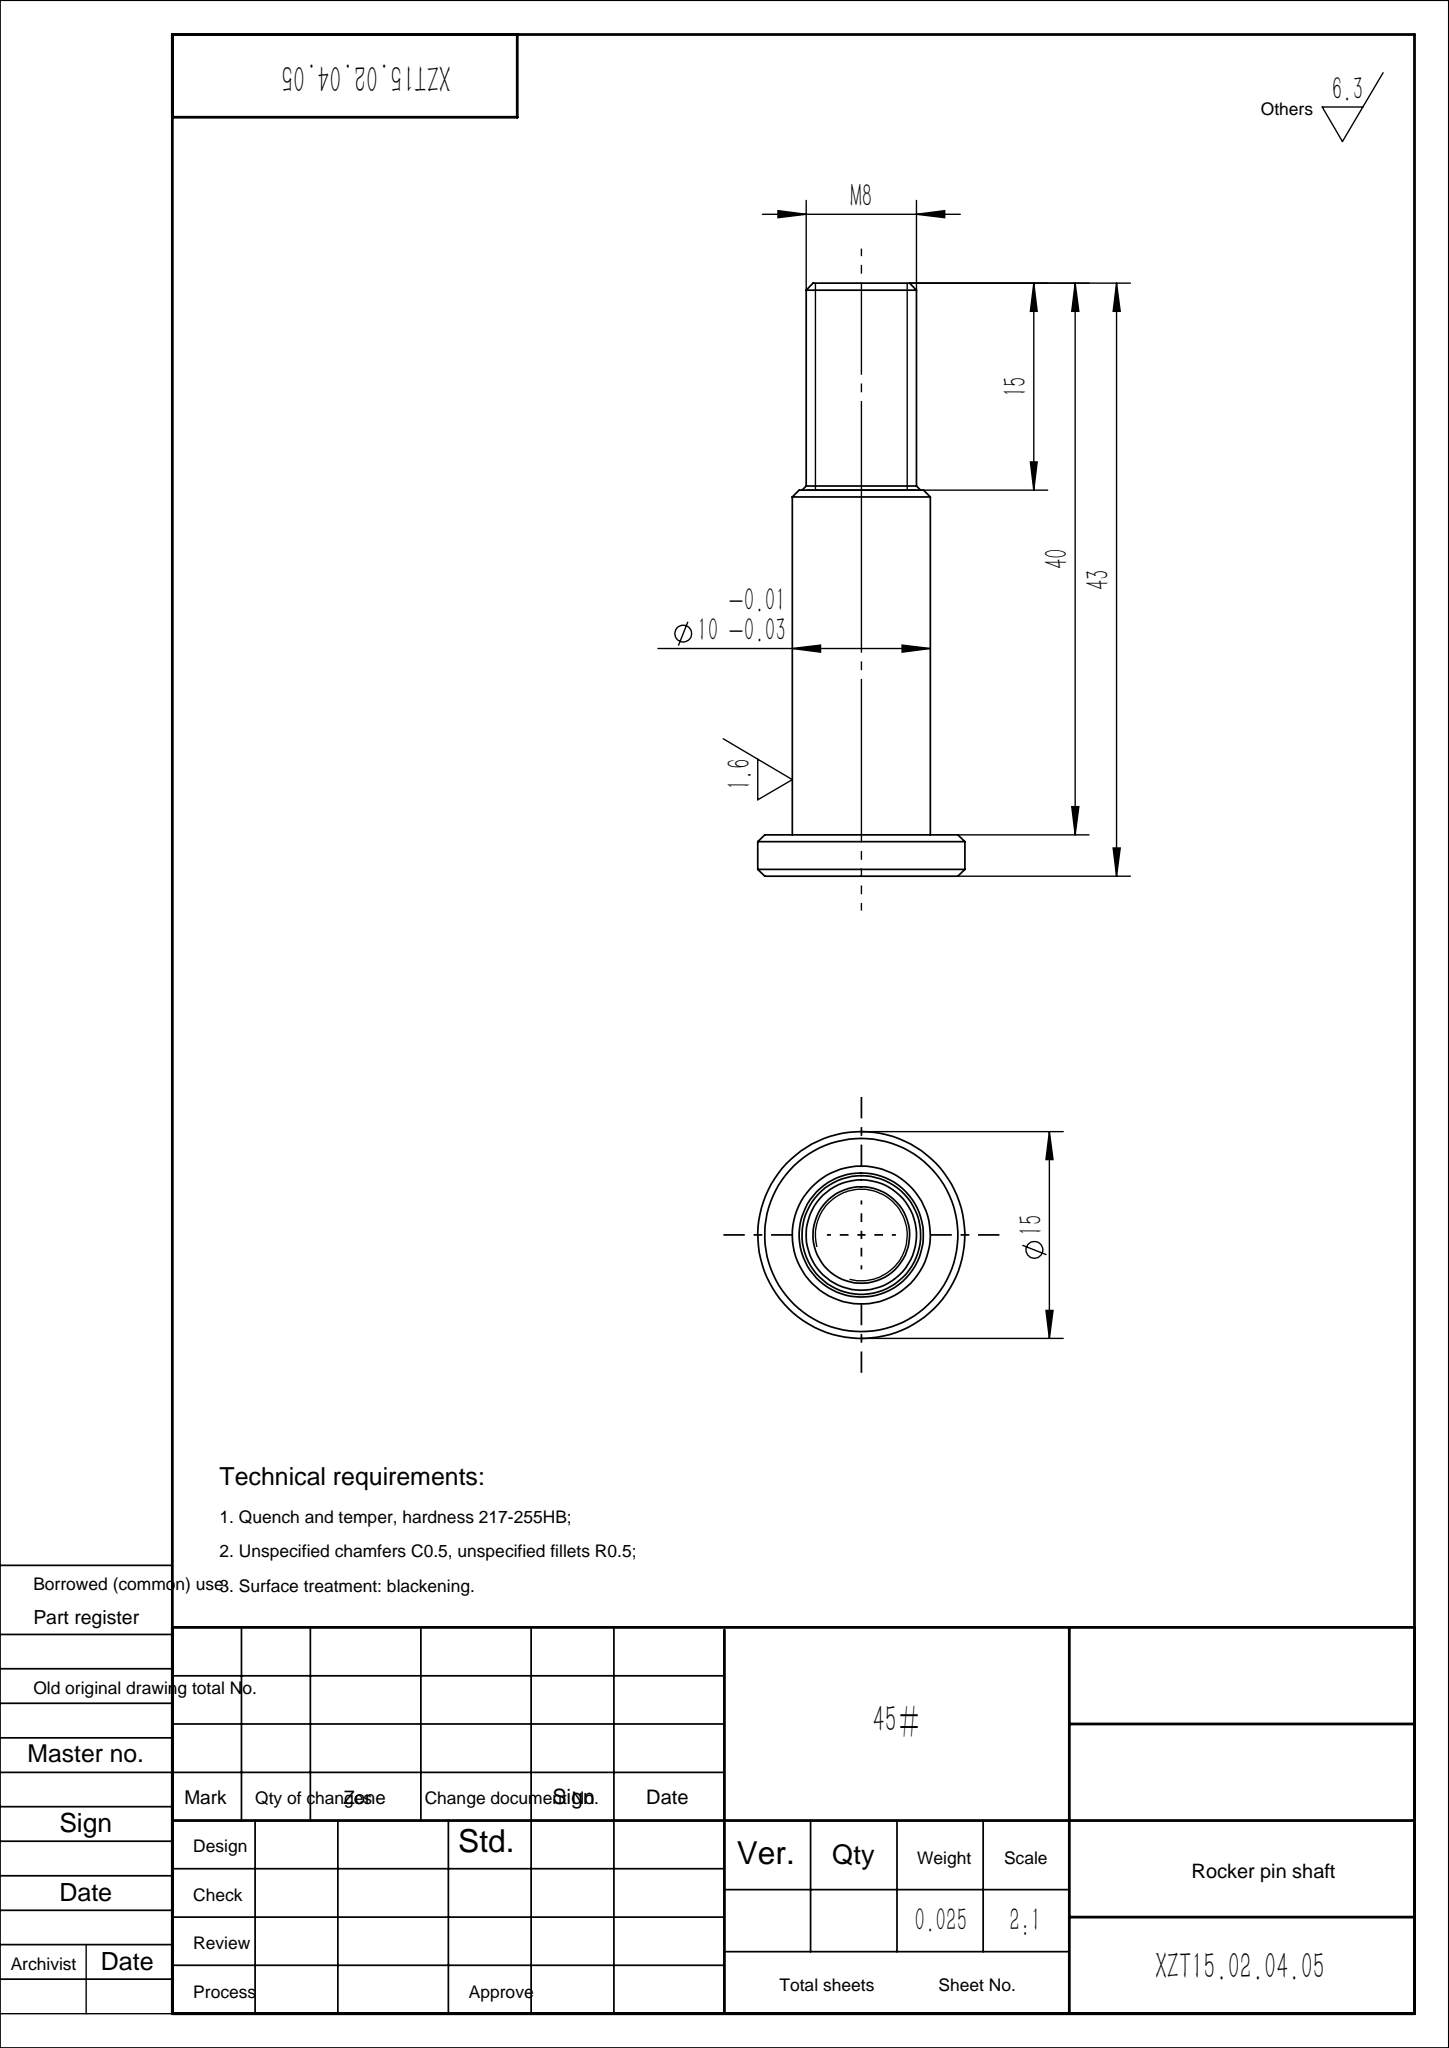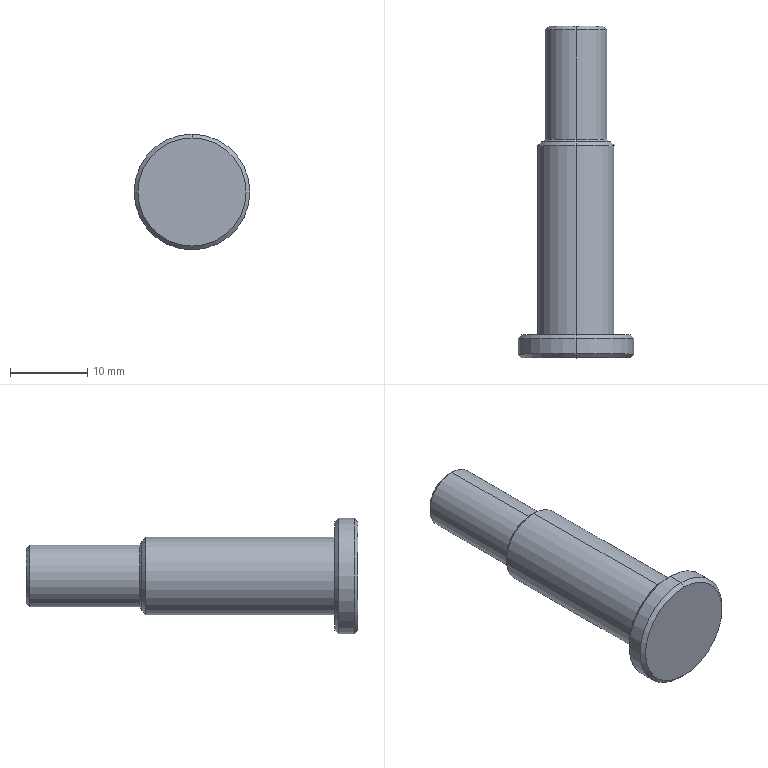Part | SolidWorks | features Chamfer 2, Revolution 1 | 1 solid | 20 faces | box 15 x 43 x 15 mm | volume 3230 mm3 | cone 10 | cylinder 6 | plane 4 | commonest cylinder face diameters 8 x2 10 x2 15 x2
STEP:
#1=CARTESIAN_POINT('',(0.,28.3,4.));
#2=VERTEX_POINT('',#1);
#3=CARTESIAN_POINT('',(0.,28.3,-4.));
#4=VERTEX_POINT('',#3);
#5=CARTESIAN_POINT('',(0.,28.3,0.));
#6=DIRECTION('',(0.,1.,0.));
#7=DIRECTION('',(0.,0.,-1.));
#8=AXIS2_PLACEMENT_3D('',#5,#6,#7);
#9=CIRCLE('',#8,4.);
#10=EDGE_CURVE('',#2,#4,#9,.T.);
#11=ORIENTED_EDGE('',*,*,#10,.F.);
#12=CARTESIAN_POINT('',(0.,28.,4.3));
#13=VERTEX_POINT('',#12);
#14=CARTESIAN_POINT('',(0.,28.3,4.));
#15=DIRECTION('',(0.,-0.7071,0.7071));
#16=VECTOR('',#15,1000.);
#17=LINE('',#14,#16);
#18=EDGE_CURVE('',#2,#13,#17,.T.);
#19=ORIENTED_EDGE('',*,*,#18,.T.);
#20=CARTESIAN_POINT('',(0.,28.,-4.3));
#21=VERTEX_POINT('',#20);
#22=CARTESIAN_POINT('',(0.,28.,0.));
#23=DIRECTION('',(0.,-1.,0.));
#24=DIRECTION('',(0.,0.,-1.));
#25=AXIS2_PLACEMENT_3D('',#22,#23,#24);
#26=CIRCLE('',#25,4.3);
#27=EDGE_CURVE('',#21,#13,#26,.T.);
#28=ORIENTED_EDGE('',*,*,#27,.F.);
#29=CARTESIAN_POINT('',(0.,28.3,-4.));
#30=DIRECTION('',(0.,-0.7071,-0.7071));
#31=VECTOR('',#30,1000.);
#32=LINE('',#29,#31);
#33=EDGE_CURVE('',#4,#21,#32,.T.);
#34=ORIENTED_EDGE('',*,*,#33,.F.);
#35=EDGE_LOOP('',(#11,#19,#28,#34));
#36=FACE_OUTER_BOUND('',#35,.T.);
#37=CARTESIAN_POINT('',(0.,28.3,0.));
#38=DIRECTION('',(0.,-1.,0.));
#39=DIRECTION('',(0.,0.,-1.));
#40=AXIS2_PLACEMENT_3D('',#37,#38,#39);
#41=CONICAL_SURFACE('',#40,4.,0.7854);
#42=ADVANCED_FACE('',(#36),#41,.T.);
#43=CARTESIAN_POINT('',(0.,28.,4.5));
#44=VERTEX_POINT('',#43);
#45=CARTESIAN_POINT('',(0.,28.,-4.5));
#46=VERTEX_POINT('',#45);
#47=CARTESIAN_POINT('',(0.,28.,0.));
#48=DIRECTION('',(0.,1.,0.));
#49=DIRECTION('',(0.,0.,-1.));
#50=AXIS2_PLACEMENT_3D('',#47,#48,#49);
#51=CIRCLE('',#50,4.5);
#52=EDGE_CURVE('',#44,#46,#51,.T.);
#53=ORIENTED_EDGE('',*,*,#52,.F.);
#54=CARTESIAN_POINT('',(0.,27.5,5.));
#55=VERTEX_POINT('',#54);
#56=CARTESIAN_POINT('',(0.,28.,4.5));
#57=DIRECTION('',(0.,-0.7071,0.7071));
#58=VECTOR('',#57,1000.);
#59=LINE('',#56,#58);
#60=EDGE_CURVE('',#44,#55,#59,.T.);
#61=ORIENTED_EDGE('',*,*,#60,.T.);
#62=CARTESIAN_POINT('',(0.,27.5,-5.));
#63=VERTEX_POINT('',#62);
#64=CARTESIAN_POINT('',(0.,27.5,0.));
#65=DIRECTION('',(0.,-1.,0.));
#66=DIRECTION('',(0.,0.,-1.));
#67=AXIS2_PLACEMENT_3D('',#64,#65,#66);
#68=CIRCLE('',#67,5.);
#69=EDGE_CURVE('',#63,#55,#68,.T.);
#70=ORIENTED_EDGE('',*,*,#69,.F.);
#71=CARTESIAN_POINT('',(0.,28.,-4.5));
#72=DIRECTION('',(0.,-0.7071,-0.7071));
#73=VECTOR('',#72,1000.);
#74=LINE('',#71,#73);
#75=EDGE_CURVE('',#46,#63,#74,.T.);
#76=ORIENTED_EDGE('',*,*,#75,.F.);
#77=EDGE_LOOP('',(#53,#61,#70,#76));
#78=FACE_OUTER_BOUND('',#77,.T.);
#79=CARTESIAN_POINT('',(0.,28.,0.));
#80=DIRECTION('',(0.,-1.,0.));
#81=DIRECTION('',(0.,0.,-1.));
#82=AXIS2_PLACEMENT_3D('',#79,#80,#81);
#83=CONICAL_SURFACE('',#82,4.5,0.7854);
#84=ADVANCED_FACE('',(#78),#83,.T.);
#85=CARTESIAN_POINT('',(0.,0.,-7.));
#86=VERTEX_POINT('',#85);
#87=CARTESIAN_POINT('',(0.,0.,7.));
#88=VERTEX_POINT('',#87);
#89=CARTESIAN_POINT('',(0.,0.,0.));
#90=DIRECTION('',(0.,-1.,0.));
#91=DIRECTION('',(0.,0.,1.));
#92=AXIS2_PLACEMENT_3D('',#89,#90,#91);
#93=CIRCLE('',#92,7.);
#94=EDGE_CURVE('',#86,#88,#93,.T.);
#95=ORIENTED_EDGE('',*,*,#94,.F.);
#96=CARTESIAN_POINT('',(0.,0.5,-7.5));
#97=VERTEX_POINT('',#96);
#98=CARTESIAN_POINT('',(0.,0.5,-7.5));
#99=DIRECTION('',(0.,0.7071,-0.7071));
#100=VECTOR('',#99,1000.);
#101=LINE('',#98,#100);
#102=EDGE_CURVE('',#86,#97,#101,.T.);
#103=ORIENTED_EDGE('',*,*,#102,.T.);
#104=CARTESIAN_POINT('',(0.,0.5,7.5));
#105=VERTEX_POINT('',#104);
#106=CARTESIAN_POINT('',(0.,0.5,0.));
#107=DIRECTION('',(0.,1.,0.));
#108=DIRECTION('',(0.,0.,1.));
#109=AXIS2_PLACEMENT_3D('',#106,#107,#108);
#110=CIRCLE('',#109,7.5);
#111=EDGE_CURVE('',#105,#97,#110,.T.);
#112=ORIENTED_EDGE('',*,*,#111,.F.);
#113=CARTESIAN_POINT('',(0.,0.5,7.5));
#114=DIRECTION('',(0.,0.7071,0.7071));
#115=VECTOR('',#114,1000.);
#116=LINE('',#113,#115);
#117=EDGE_CURVE('',#88,#105,#116,.T.);
#118=ORIENTED_EDGE('',*,*,#117,.F.);
#119=EDGE_LOOP('',(#95,#103,#112,#118));
#120=FACE_OUTER_BOUND('',#119,.T.);
#121=CARTESIAN_POINT('',(0.,0.5,0.));
#122=DIRECTION('',(0.,1.,0.));
#123=DIRECTION('',(0.,0.,1.));
#124=AXIS2_PLACEMENT_3D('',#121,#122,#123);
#125=CONICAL_SURFACE('',#124,7.5,0.7854);
#126=ADVANCED_FACE('',(#120),#125,.T.);
#127=CARTESIAN_POINT('',(0.,3.,7.));
#128=VERTEX_POINT('',#127);
#129=CARTESIAN_POINT('',(0.,3.,-7.));
#130=VERTEX_POINT('',#129);
#131=CARTESIAN_POINT('',(0.,3.,0.));
#132=DIRECTION('',(0.,1.,0.));
#133=DIRECTION('',(0.,0.,-1.));
#134=AXIS2_PLACEMENT_3D('',#131,#132,#133);
#135=CIRCLE('',#134,7.);
#136=EDGE_CURVE('',#128,#130,#135,.T.);
#137=ORIENTED_EDGE('',*,*,#136,.F.);
#138=CARTESIAN_POINT('',(0.,2.5,7.5));
#139=VERTEX_POINT('',#138);
#140=CARTESIAN_POINT('',(0.,3.,7.));
#141=DIRECTION('',(0.,-0.7071,0.7071));
#142=VECTOR('',#141,1000.);
#143=LINE('',#140,#142);
#144=EDGE_CURVE('',#128,#139,#143,.T.);
#145=ORIENTED_EDGE('',*,*,#144,.T.);
#146=CARTESIAN_POINT('',(0.,2.5,-7.5));
#147=VERTEX_POINT('',#146);
#148=CARTESIAN_POINT('',(0.,2.5,0.));
#149=DIRECTION('',(0.,-1.,0.));
#150=DIRECTION('',(0.,0.,-1.));
#151=AXIS2_PLACEMENT_3D('',#148,#149,#150);
#152=CIRCLE('',#151,7.5);
#153=EDGE_CURVE('',#147,#139,#152,.T.);
#154=ORIENTED_EDGE('',*,*,#153,.F.);
#155=CARTESIAN_POINT('',(0.,3.,-7.));
#156=DIRECTION('',(0.,-0.7071,-0.7071));
#157=VECTOR('',#156,1000.);
#158=LINE('',#155,#157);
#159=EDGE_CURVE('',#130,#147,#158,.T.);
#160=ORIENTED_EDGE('',*,*,#159,.F.);
#161=EDGE_LOOP('',(#137,#145,#154,#160));
#162=FACE_OUTER_BOUND('',#161,.T.);
#163=CARTESIAN_POINT('',(0.,3.,0.));
#164=DIRECTION('',(0.,-1.,0.));
#165=DIRECTION('',(0.,0.,-1.));
#166=AXIS2_PLACEMENT_3D('',#163,#164,#165);
#167=CONICAL_SURFACE('',#166,7.,0.7854);
#168=ADVANCED_FACE('',(#162),#167,.T.);
#169=CARTESIAN_POINT('',(0.,43.,3.5));
#170=VERTEX_POINT('',#169);
#171=CARTESIAN_POINT('',(0.,43.,-3.5));
#172=VERTEX_POINT('',#171);
#173=CARTESIAN_POINT('',(0.,43.,0.));
#174=DIRECTION('',(0.,1.,0.));
#175=DIRECTION('',(0.,0.,-1.));
#176=AXIS2_PLACEMENT_3D('',#173,#174,#175);
#177=CIRCLE('',#176,3.5);
#178=EDGE_CURVE('',#170,#172,#177,.T.);
#179=ORIENTED_EDGE('',*,*,#178,.F.);
#180=CARTESIAN_POINT('',(0.,42.5,4.));
#181=VERTEX_POINT('',#180);
#182=CARTESIAN_POINT('',(0.,43.,3.5));
#183=DIRECTION('',(0.,-0.7071,0.7071));
#184=VECTOR('',#183,1000.);
#185=LINE('',#182,#184);
#186=EDGE_CURVE('',#170,#181,#185,.T.);
#187=ORIENTED_EDGE('',*,*,#186,.T.);
#188=CARTESIAN_POINT('',(0.,42.5,-4.));
#189=VERTEX_POINT('',#188);
#190=CARTESIAN_POINT('',(0.,42.5,0.));
#191=DIRECTION('',(0.,-1.,0.));
#192=DIRECTION('',(0.,0.,-1.));
#193=AXIS2_PLACEMENT_3D('',#190,#191,#192);
#194=CIRCLE('',#193,4.);
#195=EDGE_CURVE('',#189,#181,#194,.T.);
#196=ORIENTED_EDGE('',*,*,#195,.F.);
#197=CARTESIAN_POINT('',(0.,43.,-3.5));
#198=DIRECTION('',(0.,-0.7071,-0.7071));
#199=VECTOR('',#198,1000.);
#200=LINE('',#197,#199);
#201=EDGE_CURVE('',#172,#189,#200,.T.);
#202=ORIENTED_EDGE('',*,*,#201,.F.);
#203=EDGE_LOOP('',(#179,#187,#196,#202));
#204=FACE_OUTER_BOUND('',#203,.T.);
#205=CARTESIAN_POINT('',(0.,43.,0.));
#206=DIRECTION('',(0.,-1.,0.));
#207=DIRECTION('',(0.,0.,-1.));
#208=AXIS2_PLACEMENT_3D('',#205,#206,#207);
#209=CONICAL_SURFACE('',#208,3.5,0.7854);
#210=ADVANCED_FACE('',(#204),#209,.T.);
#211=ORIENTED_EDGE('',*,*,#10,.T.);
#212=CARTESIAN_POINT('',(0.,0.,-4.));
#213=DIRECTION('',(0.,1.,0.));
#214=VECTOR('',#213,1000.);
#215=LINE('',#212,#214);
#216=EDGE_CURVE('',#4,#189,#215,.T.);
#217=ORIENTED_EDGE('',*,*,#216,.T.);
#218=ORIENTED_EDGE('',*,*,#195,.T.);
#219=CARTESIAN_POINT('',(0.,0.,4.));
#220=DIRECTION('',(0.,1.,0.));
#221=VECTOR('',#220,1000.);
#222=LINE('',#219,#221);
#223=EDGE_CURVE('',#2,#181,#222,.T.);
#224=ORIENTED_EDGE('',*,*,#223,.F.);
#225=EDGE_LOOP('',(#211,#217,#218,#224));
#226=FACE_OUTER_BOUND('',#225,.T.);
#227=CARTESIAN_POINT('',(0.,0.,0.));
#228=DIRECTION('',(0.,1.,0.));
#229=DIRECTION('',(0.,0.,1.));
#230=AXIS2_PLACEMENT_3D('',#227,#228,#229);
#231=CYLINDRICAL_SURFACE('',#230,4.);
#232=ADVANCED_FACE('',(#226),#231,.T.);
#233=CARTESIAN_POINT('',(0.,3.,5.));
#234=VERTEX_POINT('',#233);
#235=CARTESIAN_POINT('',(0.,3.,-5.));
#236=VERTEX_POINT('',#235);
#237=CARTESIAN_POINT('',(0.,3.,0.));
#238=DIRECTION('',(0.,1.,0.));
#239=DIRECTION('',(0.,0.,1.));
#240=AXIS2_PLACEMENT_3D('',#237,#238,#239);
#241=CIRCLE('',#240,5.);
#242=EDGE_CURVE('',#234,#236,#241,.T.);
#243=ORIENTED_EDGE('',*,*,#242,.T.);
#244=CARTESIAN_POINT('',(0.,0.,-5.));
#245=DIRECTION('',(0.,1.,0.));
#246=VECTOR('',#245,1000.);
#247=LINE('',#244,#246);
#248=EDGE_CURVE('',#236,#63,#247,.T.);
#249=ORIENTED_EDGE('',*,*,#248,.T.);
#250=ORIENTED_EDGE('',*,*,#69,.T.);
#251=CARTESIAN_POINT('',(0.,0.,5.));
#252=DIRECTION('',(0.,1.,0.));
#253=VECTOR('',#252,1000.);
#254=LINE('',#251,#253);
#255=EDGE_CURVE('',#234,#55,#254,.T.);
#256=ORIENTED_EDGE('',*,*,#255,.F.);
#257=EDGE_LOOP('',(#243,#249,#250,#256));
#258=FACE_OUTER_BOUND('',#257,.T.);
#259=CARTESIAN_POINT('',(0.,0.,0.));
#260=DIRECTION('',(0.,1.,0.));
#261=DIRECTION('',(0.,0.,1.));
#262=AXIS2_PLACEMENT_3D('',#259,#260,#261);
#263=CYLINDRICAL_SURFACE('',#262,5.);
#264=ADVANCED_FACE('',(#258),#263,.T.);
#265=ORIENTED_EDGE('',*,*,#111,.T.);
#266=CARTESIAN_POINT('',(0.,0.,-7.5));
#267=DIRECTION('',(0.,1.,0.));
#268=VECTOR('',#267,1000.);
#269=LINE('',#266,#268);
#270=EDGE_CURVE('',#97,#147,#269,.T.);
#271=ORIENTED_EDGE('',*,*,#270,.T.);
#272=ORIENTED_EDGE('',*,*,#153,.T.);
#273=CARTESIAN_POINT('',(0.,0.,7.5));
#274=DIRECTION('',(0.,1.,0.));
#275=VECTOR('',#274,1000.);
#276=LINE('',#273,#275);
#277=EDGE_CURVE('',#105,#139,#276,.T.);
#278=ORIENTED_EDGE('',*,*,#277,.F.);
#279=EDGE_LOOP('',(#265,#271,#272,#278));
#280=FACE_OUTER_BOUND('',#279,.T.);
#281=CARTESIAN_POINT('',(0.,0.,0.));
#282=DIRECTION('',(0.,1.,0.));
#283=DIRECTION('',(0.,0.,1.));
#284=AXIS2_PLACEMENT_3D('',#281,#282,#283);
#285=CYLINDRICAL_SURFACE('',#284,7.5);
#286=ADVANCED_FACE('',(#280),#285,.T.);
#287=CARTESIAN_POINT('',(0.,0.,0.));
#288=DIRECTION('',(0.,-1.,0.));
#289=DIRECTION('',(0.,0.,1.));
#290=AXIS2_PLACEMENT_3D('',#287,#288,#289);
#291=CIRCLE('',#290,7.);
#292=EDGE_CURVE('',#88,#86,#291,.T.);
#293=ORIENTED_EDGE('',*,*,#292,.T.);
#294=ORIENTED_EDGE('',*,*,#94,.T.);
#295=EDGE_LOOP('',(#293,#294));
#296=FACE_OUTER_BOUND('',#295,.T.);
#297=CARTESIAN_POINT('',(0.,0.,0.));
#298=DIRECTION('',(0.,1.,0.));
#299=DIRECTION('',(0.,0.,1.));
#300=AXIS2_PLACEMENT_3D('',#297,#298,#299);
#301=PLANE('',#300);
#302=ADVANCED_FACE('',(#296),#301,.F.);
#303=ORIENTED_EDGE('',*,*,#270,.F.);
#304=CARTESIAN_POINT('',(0.,0.5,0.));
#305=DIRECTION('',(0.,1.,0.));
#306=DIRECTION('',(0.,0.,1.));
#307=AXIS2_PLACEMENT_3D('',#304,#305,#306);
#308=CIRCLE('',#307,7.5);
#309=EDGE_CURVE('',#97,#105,#308,.T.);
#310=ORIENTED_EDGE('',*,*,#309,.T.);
#311=ORIENTED_EDGE('',*,*,#277,.T.);
#312=CARTESIAN_POINT('',(0.,2.5,0.));
#313=DIRECTION('',(0.,-1.,0.));
#314=DIRECTION('',(0.,0.,-1.));
#315=AXIS2_PLACEMENT_3D('',#312,#313,#314);
#316=CIRCLE('',#315,7.5);
#317=EDGE_CURVE('',#139,#147,#316,.T.);
#318=ORIENTED_EDGE('',*,*,#317,.T.);
#319=EDGE_LOOP('',(#303,#310,#311,#318));
#320=FACE_OUTER_BOUND('',#319,.T.);
#321=CARTESIAN_POINT('',(0.,0.,0.));
#322=DIRECTION('',(0.,1.,0.));
#323=DIRECTION('',(0.,0.,1.));
#324=AXIS2_PLACEMENT_3D('',#321,#322,#323);
#325=CYLINDRICAL_SURFACE('',#324,7.5);
#326=ADVANCED_FACE('',(#320),#325,.T.);
#327=CARTESIAN_POINT('',(0.,3.,0.));
#328=DIRECTION('',(0.,1.,0.));
#329=DIRECTION('',(0.,0.,-1.));
#330=AXIS2_PLACEMENT_3D('',#327,#328,#329);
#331=CIRCLE('',#330,7.);
#332=EDGE_CURVE('',#130,#128,#331,.T.);
#333=ORIENTED_EDGE('',*,*,#332,.T.);
#334=ORIENTED_EDGE('',*,*,#136,.T.);
#335=EDGE_LOOP('',(#333,#334));
#336=FACE_OUTER_BOUND('',#335,.T.);
#337=ORIENTED_EDGE('',*,*,#242,.F.);
#338=CARTESIAN_POINT('',(0.,3.,0.));
#339=DIRECTION('',(0.,1.,0.));
#340=DIRECTION('',(0.,0.,1.));
#341=AXIS2_PLACEMENT_3D('',#338,#339,#340);
#342=CIRCLE('',#341,5.);
#343=EDGE_CURVE('',#236,#234,#342,.T.);
#344=ORIENTED_EDGE('',*,*,#343,.F.);
#345=EDGE_LOOP('',(#337,#344));
#346=FACE_BOUND('',#345,.T.);
#347=CARTESIAN_POINT('',(7.5,3.,0.));
#348=DIRECTION('',(0.,-1.,0.));
#349=DIRECTION('',(0.,0.,-1.));
#350=AXIS2_PLACEMENT_3D('',#347,#348,#349);
#351=PLANE('',#350);
#352=ADVANCED_FACE('',(#336,#346),#351,.F.);
#353=ORIENTED_EDGE('',*,*,#248,.F.);
#354=ORIENTED_EDGE('',*,*,#343,.T.);
#355=ORIENTED_EDGE('',*,*,#255,.T.);
#356=CARTESIAN_POINT('',(0.,27.5,0.));
#357=DIRECTION('',(0.,-1.,0.));
#358=DIRECTION('',(0.,0.,-1.));
#359=AXIS2_PLACEMENT_3D('',#356,#357,#358);
#360=CIRCLE('',#359,5.);
#361=EDGE_CURVE('',#55,#63,#360,.T.);
#362=ORIENTED_EDGE('',*,*,#361,.T.);
#363=EDGE_LOOP('',(#353,#354,#355,#362));
#364=FACE_OUTER_BOUND('',#363,.T.);
#365=CARTESIAN_POINT('',(0.,0.,0.));
#366=DIRECTION('',(0.,1.,0.));
#367=DIRECTION('',(0.,0.,1.));
#368=AXIS2_PLACEMENT_3D('',#365,#366,#367);
#369=CYLINDRICAL_SURFACE('',#368,5.);
#370=ADVANCED_FACE('',(#364),#369,.T.);
#371=ORIENTED_EDGE('',*,*,#27,.T.);
#372=CARTESIAN_POINT('',(0.,28.,0.));
#373=DIRECTION('',(0.,-1.,0.));
#374=DIRECTION('',(0.,0.,-1.));
#375=AXIS2_PLACEMENT_3D('',#372,#373,#374);
#376=CIRCLE('',#375,4.3);
#377=EDGE_CURVE('',#13,#21,#376,.T.);
#378=ORIENTED_EDGE('',*,*,#377,.T.);
#379=EDGE_LOOP('',(#371,#378));
#380=FACE_BOUND('',#379,.T.);
#381=CARTESIAN_POINT('',(0.,28.,0.));
#382=DIRECTION('',(0.,1.,0.));
#383=DIRECTION('',(0.,0.,-1.));
#384=AXIS2_PLACEMENT_3D('',#381,#382,#383);
#385=CIRCLE('',#384,4.5);
#386=EDGE_CURVE('',#46,#44,#385,.T.);
#387=ORIENTED_EDGE('',*,*,#386,.T.);
#388=ORIENTED_EDGE('',*,*,#52,.T.);
#389=EDGE_LOOP('',(#387,#388));
#390=FACE_OUTER_BOUND('',#389,.T.);
#391=CARTESIAN_POINT('',(5.,28.,0.));
#392=DIRECTION('',(0.,-1.,0.));
#393=DIRECTION('',(0.,0.,-1.));
#394=AXIS2_PLACEMENT_3D('',#391,#392,#393);
#395=PLANE('',#394);
#396=ADVANCED_FACE('',(#380,#390),#395,.F.);
#397=ORIENTED_EDGE('',*,*,#216,.F.);
#398=CARTESIAN_POINT('',(0.,28.3,0.));
#399=DIRECTION('',(0.,1.,0.));
#400=DIRECTION('',(0.,0.,-1.));
#401=AXIS2_PLACEMENT_3D('',#398,#399,#400);
#402=CIRCLE('',#401,4.);
#403=EDGE_CURVE('',#4,#2,#402,.T.);
#404=ORIENTED_EDGE('',*,*,#403,.T.);
#405=ORIENTED_EDGE('',*,*,#223,.T.);
#406=CARTESIAN_POINT('',(0.,42.5,0.));
#407=DIRECTION('',(0.,-1.,0.));
#408=DIRECTION('',(0.,0.,-1.));
#409=AXIS2_PLACEMENT_3D('',#406,#407,#408);
#410=CIRCLE('',#409,4.);
#411=EDGE_CURVE('',#181,#189,#410,.T.);
#412=ORIENTED_EDGE('',*,*,#411,.T.);
#413=EDGE_LOOP('',(#397,#404,#405,#412));
#414=FACE_OUTER_BOUND('',#413,.T.);
#415=CARTESIAN_POINT('',(0.,0.,0.));
#416=DIRECTION('',(0.,1.,0.));
#417=DIRECTION('',(0.,0.,1.));
#418=AXIS2_PLACEMENT_3D('',#415,#416,#417);
#419=CYLINDRICAL_SURFACE('',#418,4.);
#420=ADVANCED_FACE('',(#414),#419,.T.);
#421=CARTESIAN_POINT('',(0.,43.,0.));
#422=DIRECTION('',(0.,1.,0.));
#423=DIRECTION('',(0.,0.,-1.));
#424=AXIS2_PLACEMENT_3D('',#421,#422,#423);
#425=CIRCLE('',#424,3.5);
#426=EDGE_CURVE('',#172,#170,#425,.T.);
#427=ORIENTED_EDGE('',*,*,#426,.T.);
#428=ORIENTED_EDGE('',*,*,#178,.T.);
#429=EDGE_LOOP('',(#427,#428));
#430=FACE_OUTER_BOUND('',#429,.T.);
#431=CARTESIAN_POINT('',(4.,43.,0.));
#432=DIRECTION('',(0.,-1.,0.));
#433=DIRECTION('',(0.,0.,-1.));
#434=AXIS2_PLACEMENT_3D('',#431,#432,#433);
#435=PLANE('',#434);
#436=ADVANCED_FACE('',(#430),#435,.F.);
#437=ORIENTED_EDGE('',*,*,#186,.F.);
#438=ORIENTED_EDGE('',*,*,#426,.F.);
#439=ORIENTED_EDGE('',*,*,#201,.T.);
#440=ORIENTED_EDGE('',*,*,#411,.F.);
#441=EDGE_LOOP('',(#437,#438,#439,#440));
#442=FACE_OUTER_BOUND('',#441,.T.);
#443=CARTESIAN_POINT('',(0.,43.,0.));
#444=DIRECTION('',(0.,-1.,0.));
#445=DIRECTION('',(0.,0.,-1.));
#446=AXIS2_PLACEMENT_3D('',#443,#444,#445);
#447=CONICAL_SURFACE('',#446,3.5,0.7854);
#448=ADVANCED_FACE('',(#442),#447,.T.);
#449=ORIENTED_EDGE('',*,*,#144,.F.);
#450=ORIENTED_EDGE('',*,*,#332,.F.);
#451=ORIENTED_EDGE('',*,*,#159,.T.);
#452=ORIENTED_EDGE('',*,*,#317,.F.);
#453=EDGE_LOOP('',(#449,#450,#451,#452));
#454=FACE_OUTER_BOUND('',#453,.T.);
#455=CARTESIAN_POINT('',(0.,3.,0.));
#456=DIRECTION('',(0.,-1.,0.));
#457=DIRECTION('',(0.,0.,-1.));
#458=AXIS2_PLACEMENT_3D('',#455,#456,#457);
#459=CONICAL_SURFACE('',#458,7.,0.7854);
#460=ADVANCED_FACE('',(#454),#459,.T.);
#461=ORIENTED_EDGE('',*,*,#102,.F.);
#462=ORIENTED_EDGE('',*,*,#292,.F.);
#463=ORIENTED_EDGE('',*,*,#117,.T.);
#464=ORIENTED_EDGE('',*,*,#309,.F.);
#465=EDGE_LOOP('',(#461,#462,#463,#464));
#466=FACE_OUTER_BOUND('',#465,.T.);
#467=CARTESIAN_POINT('',(0.,0.5,0.));
#468=DIRECTION('',(0.,1.,0.));
#469=DIRECTION('',(0.,0.,1.));
#470=AXIS2_PLACEMENT_3D('',#467,#468,#469);
#471=CONICAL_SURFACE('',#470,7.5,0.7854);
#472=ADVANCED_FACE('',(#466),#471,.T.);
#473=ORIENTED_EDGE('',*,*,#60,.F.);
#474=ORIENTED_EDGE('',*,*,#386,.F.);
#475=ORIENTED_EDGE('',*,*,#75,.T.);
#476=ORIENTED_EDGE('',*,*,#361,.F.);
#477=EDGE_LOOP('',(#473,#474,#475,#476));
#478=FACE_OUTER_BOUND('',#477,.T.);
#479=CARTESIAN_POINT('',(0.,28.,0.));
#480=DIRECTION('',(0.,-1.,0.));
#481=DIRECTION('',(0.,0.,-1.));
#482=AXIS2_PLACEMENT_3D('',#479,#480,#481);
#483=CONICAL_SURFACE('',#482,4.5,0.7854);
#484=ADVANCED_FACE('',(#478),#483,.T.);
#485=ORIENTED_EDGE('',*,*,#18,.F.);
#486=ORIENTED_EDGE('',*,*,#403,.F.);
#487=ORIENTED_EDGE('',*,*,#33,.T.);
#488=ORIENTED_EDGE('',*,*,#377,.F.);
#489=EDGE_LOOP('',(#485,#486,#487,#488));
#490=FACE_OUTER_BOUND('',#489,.T.);
#491=CARTESIAN_POINT('',(0.,28.3,0.));
#492=DIRECTION('',(0.,-1.,0.));
#493=DIRECTION('',(0.,0.,-1.));
#494=AXIS2_PLACEMENT_3D('',#491,#492,#493);
#495=CONICAL_SURFACE('',#494,4.,0.7854);
#496=ADVANCED_FACE('',(#490),#495,.T.);
#497=CLOSED_SHELL('',(#42,#84,#126,#168,#210,#232,#264,#286,#302,#326,#352,#370,#396,#420,#436,#448,#460,#472,#484,#496));
#498=MANIFOLD_SOLID_BREP('',#497);
#499=CARTESIAN_POINT('',(0.,0.,0.));
#500=DIRECTION('',(0.,0.,1.));
#501=DIRECTION('',(1.,0.,0.));
#502=AXIS2_PLACEMENT_3D('',#499,#500,#501);
#503=(LENGTH_UNIT()NAMED_UNIT(*)SI_UNIT(.MILLI.,.METRE.));
#504=UNCERTAINTY_MEASURE_WITH_UNIT(LENGTH_MEASURE(0.00001),#503,'','');
#505=(NAMED_UNIT(*)PLANE_ANGLE_UNIT()SI_UNIT($,.RADIAN.));
#506=(NAMED_UNIT(*)SI_UNIT($,.STERADIAN.)SOLID_ANGLE_UNIT());
#507=(GEOMETRIC_REPRESENTATION_CONTEXT(3)GLOBAL_UNCERTAINTY_ASSIGNED_CONTEXT((#504))GLOBAL_UNIT_ASSIGNED_CONTEXT((#503,#505,#506))REPRESENTATION_CONTEXT('',''));
#508=ADVANCED_BREP_SHAPE_REPRESENTATION('',(#498,#502),#507);